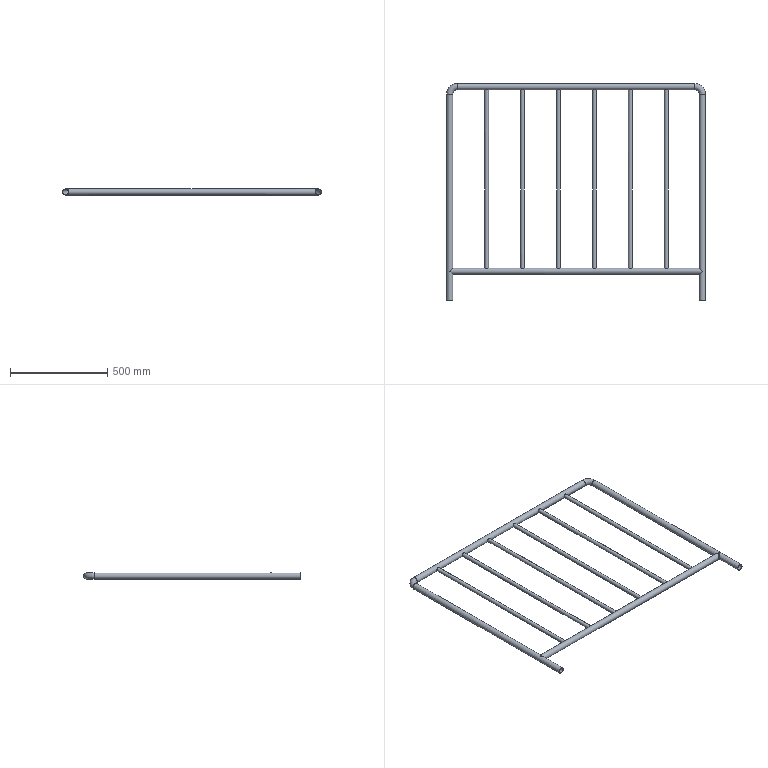Part | STEP file | 304 guardrail 1300X1100 body-B_Default<As Machined> | 12 solids | 48 faces | box 1332 x 1116 x 32 mm | volume 1011632 mm3 | cylinder 34 | plane 10 | torus 4 | commonest cylinder face diameters 32 x18 18 x6 20 x6 29 x4